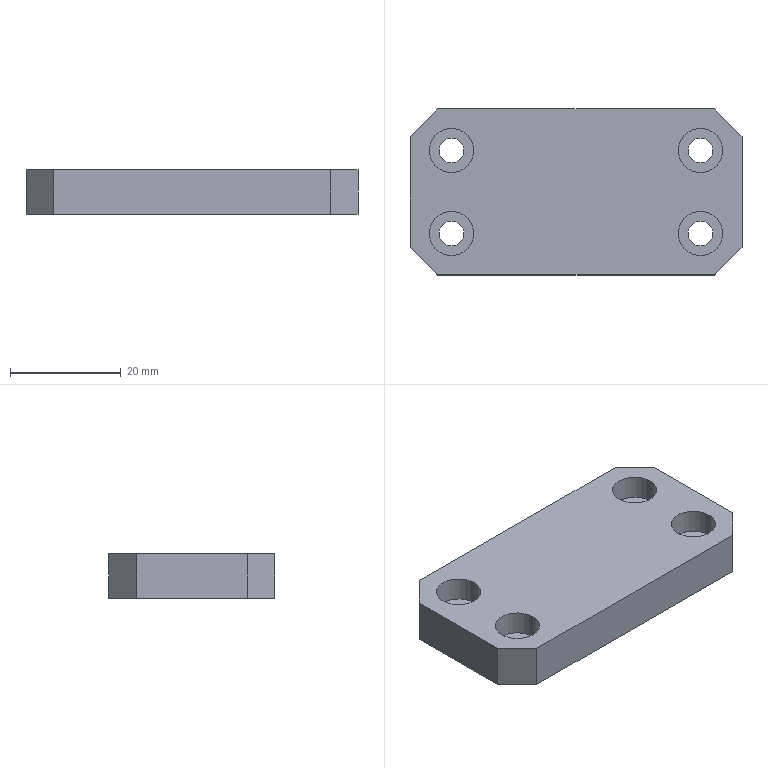Part | SolidWorks | features Chamfer 1, Extrusion 1, HoleWzd 1 | 1 solid | 30 faces | box 60 x 30 x 8 mm | volume 12886 mm3 | cylinder 16 | plane 14 | commonest cylinder face diameters 4.5 x8 8 x8
STEP:
#1=CARTESIAN_POINT('',(-26.5,7.5,3.6));
#2=VERTEX_POINT('',#1);
#3=CARTESIAN_POINT('',(-18.5,7.5,3.6));
#4=VERTEX_POINT('',#3);
#5=CARTESIAN_POINT('',(-22.5,7.5,3.6));
#6=DIRECTION('',(0.,0.,1.));
#7=DIRECTION('',(1.,0.,0.));
#8=AXIS2_PLACEMENT_3D('',#5,#6,#7);
#9=CIRCLE('',#8,4.);
#10=EDGE_CURVE('',#2,#4,#9,.T.);
#11=ORIENTED_EDGE('',*,*,#10,.F.);
#12=CARTESIAN_POINT('',(-26.5,7.5,8.));
#13=VERTEX_POINT('',#12);
#14=CARTESIAN_POINT('',(-26.5,7.5,8.));
#15=DIRECTION('',(0.,0.,1.));
#16=VECTOR('',#15,1000.);
#17=LINE('',#14,#16);
#18=EDGE_CURVE('',#2,#13,#17,.T.);
#19=ORIENTED_EDGE('',*,*,#18,.T.);
#20=CARTESIAN_POINT('',(-18.5,7.5,8.));
#21=VERTEX_POINT('',#20);
#22=CARTESIAN_POINT('',(-22.5,7.5,8.));
#23=DIRECTION('',(0.,0.,1.));
#24=DIRECTION('',(1.,0.,0.));
#25=AXIS2_PLACEMENT_3D('',#22,#23,#24);
#26=CIRCLE('',#25,4.);
#27=EDGE_CURVE('',#13,#21,#26,.T.);
#28=ORIENTED_EDGE('',*,*,#27,.T.);
#29=CARTESIAN_POINT('',(-18.5,7.5,8.));
#30=DIRECTION('',(0.,0.,1.));
#31=VECTOR('',#30,1000.);
#32=LINE('',#29,#31);
#33=EDGE_CURVE('',#4,#21,#32,.T.);
#34=ORIENTED_EDGE('',*,*,#33,.F.);
#35=EDGE_LOOP('',(#11,#19,#28,#34));
#36=FACE_OUTER_BOUND('',#35,.T.);
#37=CARTESIAN_POINT('',(-22.5,7.5,8.));
#38=DIRECTION('',(0.,0.,1.));
#39=DIRECTION('',(1.,0.,0.));
#40=AXIS2_PLACEMENT_3D('',#37,#38,#39);
#41=CYLINDRICAL_SURFACE('',#40,4.);
#42=ADVANCED_FACE('',(#36),#41,.F.);
#43=CARTESIAN_POINT('',(-24.75,7.5,0.));
#44=VERTEX_POINT('',#43);
#45=CARTESIAN_POINT('',(-20.25,7.5,0.));
#46=VERTEX_POINT('',#45);
#47=CARTESIAN_POINT('',(-22.5,7.5,0.));
#48=DIRECTION('',(0.,0.,1.));
#49=DIRECTION('',(1.,0.,0.));
#50=AXIS2_PLACEMENT_3D('',#47,#48,#49);
#51=CIRCLE('',#50,2.25);
#52=EDGE_CURVE('',#44,#46,#51,.T.);
#53=ORIENTED_EDGE('',*,*,#52,.F.);
#54=CARTESIAN_POINT('',(-24.75,7.5,3.6));
#55=VERTEX_POINT('',#54);
#56=CARTESIAN_POINT('',(-24.75,7.5,8.));
#57=DIRECTION('',(0.,0.,1.));
#58=VECTOR('',#57,1000.);
#59=LINE('',#56,#58);
#60=EDGE_CURVE('',#44,#55,#59,.T.);
#61=ORIENTED_EDGE('',*,*,#60,.T.);
#62=CARTESIAN_POINT('',(-20.25,7.5,3.6));
#63=VERTEX_POINT('',#62);
#64=CARTESIAN_POINT('',(-22.5,7.5,3.6));
#65=DIRECTION('',(0.,0.,1.));
#66=DIRECTION('',(1.,0.,0.));
#67=AXIS2_PLACEMENT_3D('',#64,#65,#66);
#68=CIRCLE('',#67,2.25);
#69=EDGE_CURVE('',#55,#63,#68,.T.);
#70=ORIENTED_EDGE('',*,*,#69,.T.);
#71=CARTESIAN_POINT('',(-20.25,7.5,8.));
#72=DIRECTION('',(0.,0.,1.));
#73=VECTOR('',#72,1000.);
#74=LINE('',#71,#73);
#75=EDGE_CURVE('',#46,#63,#74,.T.);
#76=ORIENTED_EDGE('',*,*,#75,.F.);
#77=EDGE_LOOP('',(#53,#61,#70,#76));
#78=FACE_OUTER_BOUND('',#77,.T.);
#79=CARTESIAN_POINT('',(-22.5,7.5,8.));
#80=DIRECTION('',(0.,0.,1.));
#81=DIRECTION('',(1.,0.,0.));
#82=AXIS2_PLACEMENT_3D('',#79,#80,#81);
#83=CYLINDRICAL_SURFACE('',#82,2.25);
#84=ADVANCED_FACE('',(#78),#83,.F.);
#85=CARTESIAN_POINT('',(-26.5,-7.5,3.6));
#86=VERTEX_POINT('',#85);
#87=CARTESIAN_POINT('',(-18.5,-7.5,3.6));
#88=VERTEX_POINT('',#87);
#89=CARTESIAN_POINT('',(-22.5,-7.5,3.6));
#90=DIRECTION('',(0.,0.,1.));
#91=DIRECTION('',(1.,0.,0.));
#92=AXIS2_PLACEMENT_3D('',#89,#90,#91);
#93=CIRCLE('',#92,4.);
#94=EDGE_CURVE('',#86,#88,#93,.T.);
#95=ORIENTED_EDGE('',*,*,#94,.F.);
#96=CARTESIAN_POINT('',(-26.5,-7.5,8.));
#97=VERTEX_POINT('',#96);
#98=CARTESIAN_POINT('',(-26.5,-7.5,8.));
#99=DIRECTION('',(0.,0.,1.));
#100=VECTOR('',#99,1000.);
#101=LINE('',#98,#100);
#102=EDGE_CURVE('',#86,#97,#101,.T.);
#103=ORIENTED_EDGE('',*,*,#102,.T.);
#104=CARTESIAN_POINT('',(-18.5,-7.5,8.));
#105=VERTEX_POINT('',#104);
#106=CARTESIAN_POINT('',(-22.5,-7.5,8.));
#107=DIRECTION('',(0.,0.,1.));
#108=DIRECTION('',(1.,0.,0.));
#109=AXIS2_PLACEMENT_3D('',#106,#107,#108);
#110=CIRCLE('',#109,4.);
#111=EDGE_CURVE('',#97,#105,#110,.T.);
#112=ORIENTED_EDGE('',*,*,#111,.T.);
#113=CARTESIAN_POINT('',(-18.5,-7.5,8.));
#114=DIRECTION('',(0.,0.,1.));
#115=VECTOR('',#114,1000.);
#116=LINE('',#113,#115);
#117=EDGE_CURVE('',#88,#105,#116,.T.);
#118=ORIENTED_EDGE('',*,*,#117,.F.);
#119=EDGE_LOOP('',(#95,#103,#112,#118));
#120=FACE_OUTER_BOUND('',#119,.T.);
#121=CARTESIAN_POINT('',(-22.5,-7.5,8.));
#122=DIRECTION('',(0.,0.,1.));
#123=DIRECTION('',(1.,0.,0.));
#124=AXIS2_PLACEMENT_3D('',#121,#122,#123);
#125=CYLINDRICAL_SURFACE('',#124,4.);
#126=ADVANCED_FACE('',(#120),#125,.F.);
#127=CARTESIAN_POINT('',(-24.75,-7.5,0.));
#128=VERTEX_POINT('',#127);
#129=CARTESIAN_POINT('',(-20.25,-7.5,0.));
#130=VERTEX_POINT('',#129);
#131=CARTESIAN_POINT('',(-22.5,-7.5,0.));
#132=DIRECTION('',(0.,0.,1.));
#133=DIRECTION('',(1.,0.,0.));
#134=AXIS2_PLACEMENT_3D('',#131,#132,#133);
#135=CIRCLE('',#134,2.25);
#136=EDGE_CURVE('',#128,#130,#135,.T.);
#137=ORIENTED_EDGE('',*,*,#136,.F.);
#138=CARTESIAN_POINT('',(-24.75,-7.5,3.6));
#139=VERTEX_POINT('',#138);
#140=CARTESIAN_POINT('',(-24.75,-7.5,8.));
#141=DIRECTION('',(0.,0.,1.));
#142=VECTOR('',#141,1000.);
#143=LINE('',#140,#142);
#144=EDGE_CURVE('',#128,#139,#143,.T.);
#145=ORIENTED_EDGE('',*,*,#144,.T.);
#146=CARTESIAN_POINT('',(-20.25,-7.5,3.6));
#147=VERTEX_POINT('',#146);
#148=CARTESIAN_POINT('',(-22.5,-7.5,3.6));
#149=DIRECTION('',(0.,0.,1.));
#150=DIRECTION('',(1.,0.,0.));
#151=AXIS2_PLACEMENT_3D('',#148,#149,#150);
#152=CIRCLE('',#151,2.25);
#153=EDGE_CURVE('',#139,#147,#152,.T.);
#154=ORIENTED_EDGE('',*,*,#153,.T.);
#155=CARTESIAN_POINT('',(-20.25,-7.5,8.));
#156=DIRECTION('',(0.,0.,1.));
#157=VECTOR('',#156,1000.);
#158=LINE('',#155,#157);
#159=EDGE_CURVE('',#130,#147,#158,.T.);
#160=ORIENTED_EDGE('',*,*,#159,.F.);
#161=EDGE_LOOP('',(#137,#145,#154,#160));
#162=FACE_OUTER_BOUND('',#161,.T.);
#163=CARTESIAN_POINT('',(-22.5,-7.5,8.));
#164=DIRECTION('',(0.,0.,1.));
#165=DIRECTION('',(1.,0.,0.));
#166=AXIS2_PLACEMENT_3D('',#163,#164,#165);
#167=CYLINDRICAL_SURFACE('',#166,2.25);
#168=ADVANCED_FACE('',(#162),#167,.F.);
#169=CARTESIAN_POINT('',(18.5,-7.5,3.6));
#170=VERTEX_POINT('',#169);
#171=CARTESIAN_POINT('',(26.5,-7.5,3.6));
#172=VERTEX_POINT('',#171);
#173=CARTESIAN_POINT('',(22.5,-7.5,3.6));
#174=DIRECTION('',(0.,0.,1.));
#175=DIRECTION('',(1.,0.,0.));
#176=AXIS2_PLACEMENT_3D('',#173,#174,#175);
#177=CIRCLE('',#176,4.);
#178=EDGE_CURVE('',#170,#172,#177,.T.);
#179=ORIENTED_EDGE('',*,*,#178,.F.);
#180=CARTESIAN_POINT('',(18.5,-7.5,8.));
#181=VERTEX_POINT('',#180);
#182=CARTESIAN_POINT('',(18.5,-7.5,8.));
#183=DIRECTION('',(0.,0.,1.));
#184=VECTOR('',#183,1000.);
#185=LINE('',#182,#184);
#186=EDGE_CURVE('',#170,#181,#185,.T.);
#187=ORIENTED_EDGE('',*,*,#186,.T.);
#188=CARTESIAN_POINT('',(26.5,-7.5,8.));
#189=VERTEX_POINT('',#188);
#190=CARTESIAN_POINT('',(22.5,-7.5,8.));
#191=DIRECTION('',(0.,0.,1.));
#192=DIRECTION('',(1.,0.,0.));
#193=AXIS2_PLACEMENT_3D('',#190,#191,#192);
#194=CIRCLE('',#193,4.);
#195=EDGE_CURVE('',#181,#189,#194,.T.);
#196=ORIENTED_EDGE('',*,*,#195,.T.);
#197=CARTESIAN_POINT('',(26.5,-7.5,8.));
#198=DIRECTION('',(0.,0.,1.));
#199=VECTOR('',#198,1000.);
#200=LINE('',#197,#199);
#201=EDGE_CURVE('',#172,#189,#200,.T.);
#202=ORIENTED_EDGE('',*,*,#201,.F.);
#203=EDGE_LOOP('',(#179,#187,#196,#202));
#204=FACE_OUTER_BOUND('',#203,.T.);
#205=CARTESIAN_POINT('',(22.5,-7.5,8.));
#206=DIRECTION('',(0.,0.,1.));
#207=DIRECTION('',(1.,0.,0.));
#208=AXIS2_PLACEMENT_3D('',#205,#206,#207);
#209=CYLINDRICAL_SURFACE('',#208,4.);
#210=ADVANCED_FACE('',(#204),#209,.F.);
#211=CARTESIAN_POINT('',(20.25,-7.5,0.));
#212=VERTEX_POINT('',#211);
#213=CARTESIAN_POINT('',(24.75,-7.5,0.));
#214=VERTEX_POINT('',#213);
#215=CARTESIAN_POINT('',(22.5,-7.5,0.));
#216=DIRECTION('',(0.,0.,1.));
#217=DIRECTION('',(1.,0.,0.));
#218=AXIS2_PLACEMENT_3D('',#215,#216,#217);
#219=CIRCLE('',#218,2.25);
#220=EDGE_CURVE('',#212,#214,#219,.T.);
#221=ORIENTED_EDGE('',*,*,#220,.F.);
#222=CARTESIAN_POINT('',(20.25,-7.5,3.6));
#223=VERTEX_POINT('',#222);
#224=CARTESIAN_POINT('',(20.25,-7.5,8.));
#225=DIRECTION('',(0.,0.,1.));
#226=VECTOR('',#225,1000.);
#227=LINE('',#224,#226);
#228=EDGE_CURVE('',#212,#223,#227,.T.);
#229=ORIENTED_EDGE('',*,*,#228,.T.);
#230=CARTESIAN_POINT('',(24.75,-7.5,3.6));
#231=VERTEX_POINT('',#230);
#232=CARTESIAN_POINT('',(22.5,-7.5,3.6));
#233=DIRECTION('',(0.,0.,1.));
#234=DIRECTION('',(1.,0.,0.));
#235=AXIS2_PLACEMENT_3D('',#232,#233,#234);
#236=CIRCLE('',#235,2.25);
#237=EDGE_CURVE('',#223,#231,#236,.T.);
#238=ORIENTED_EDGE('',*,*,#237,.T.);
#239=CARTESIAN_POINT('',(24.75,-7.5,8.));
#240=DIRECTION('',(0.,0.,1.));
#241=VECTOR('',#240,1000.);
#242=LINE('',#239,#241);
#243=EDGE_CURVE('',#214,#231,#242,.T.);
#244=ORIENTED_EDGE('',*,*,#243,.F.);
#245=EDGE_LOOP('',(#221,#229,#238,#244));
#246=FACE_OUTER_BOUND('',#245,.T.);
#247=CARTESIAN_POINT('',(22.5,-7.5,8.));
#248=DIRECTION('',(0.,0.,1.));
#249=DIRECTION('',(1.,0.,0.));
#250=AXIS2_PLACEMENT_3D('',#247,#248,#249);
#251=CYLINDRICAL_SURFACE('',#250,2.25);
#252=ADVANCED_FACE('',(#246),#251,.F.);
#253=CARTESIAN_POINT('',(18.5,7.5,3.6));
#254=VERTEX_POINT('',#253);
#255=CARTESIAN_POINT('',(26.5,7.5,3.6));
#256=VERTEX_POINT('',#255);
#257=CARTESIAN_POINT('',(22.5,7.5,3.6));
#258=DIRECTION('',(0.,0.,1.));
#259=DIRECTION('',(1.,0.,0.));
#260=AXIS2_PLACEMENT_3D('',#257,#258,#259);
#261=CIRCLE('',#260,4.);
#262=EDGE_CURVE('',#254,#256,#261,.T.);
#263=ORIENTED_EDGE('',*,*,#262,.F.);
#264=CARTESIAN_POINT('',(18.5,7.5,8.));
#265=VERTEX_POINT('',#264);
#266=CARTESIAN_POINT('',(18.5,7.5,8.));
#267=DIRECTION('',(0.,0.,1.));
#268=VECTOR('',#267,1000.);
#269=LINE('',#266,#268);
#270=EDGE_CURVE('',#254,#265,#269,.T.);
#271=ORIENTED_EDGE('',*,*,#270,.T.);
#272=CARTESIAN_POINT('',(26.5,7.5,8.));
#273=VERTEX_POINT('',#272);
#274=CARTESIAN_POINT('',(22.5,7.5,8.));
#275=DIRECTION('',(0.,0.,1.));
#276=DIRECTION('',(1.,0.,0.));
#277=AXIS2_PLACEMENT_3D('',#274,#275,#276);
#278=CIRCLE('',#277,4.);
#279=EDGE_CURVE('',#265,#273,#278,.T.);
#280=ORIENTED_EDGE('',*,*,#279,.T.);
#281=CARTESIAN_POINT('',(26.5,7.5,8.));
#282=DIRECTION('',(0.,0.,1.));
#283=VECTOR('',#282,1000.);
#284=LINE('',#281,#283);
#285=EDGE_CURVE('',#256,#273,#284,.T.);
#286=ORIENTED_EDGE('',*,*,#285,.F.);
#287=EDGE_LOOP('',(#263,#271,#280,#286));
#288=FACE_OUTER_BOUND('',#287,.T.);
#289=CARTESIAN_POINT('',(22.5,7.5,8.));
#290=DIRECTION('',(0.,0.,1.));
#291=DIRECTION('',(1.,0.,0.));
#292=AXIS2_PLACEMENT_3D('',#289,#290,#291);
#293=CYLINDRICAL_SURFACE('',#292,4.);
#294=ADVANCED_FACE('',(#288),#293,.F.);
#295=CARTESIAN_POINT('',(20.25,7.5,0.));
#296=VERTEX_POINT('',#295);
#297=CARTESIAN_POINT('',(24.75,7.5,0.));
#298=VERTEX_POINT('',#297);
#299=CARTESIAN_POINT('',(22.5,7.5,0.));
#300=DIRECTION('',(0.,0.,1.));
#301=DIRECTION('',(1.,0.,0.));
#302=AXIS2_PLACEMENT_3D('',#299,#300,#301);
#303=CIRCLE('',#302,2.25);
#304=EDGE_CURVE('',#296,#298,#303,.T.);
#305=ORIENTED_EDGE('',*,*,#304,.F.);
#306=CARTESIAN_POINT('',(20.25,7.5,3.6));
#307=VERTEX_POINT('',#306);
#308=CARTESIAN_POINT('',(20.25,7.5,8.));
#309=DIRECTION('',(0.,0.,1.));
#310=VECTOR('',#309,1000.);
#311=LINE('',#308,#310);
#312=EDGE_CURVE('',#296,#307,#311,.T.);
#313=ORIENTED_EDGE('',*,*,#312,.T.);
#314=CARTESIAN_POINT('',(24.75,7.5,3.6));
#315=VERTEX_POINT('',#314);
#316=CARTESIAN_POINT('',(22.5,7.5,3.6));
#317=DIRECTION('',(0.,0.,1.));
#318=DIRECTION('',(1.,0.,0.));
#319=AXIS2_PLACEMENT_3D('',#316,#317,#318);
#320=CIRCLE('',#319,2.25);
#321=EDGE_CURVE('',#307,#315,#320,.T.);
#322=ORIENTED_EDGE('',*,*,#321,.T.);
#323=CARTESIAN_POINT('',(24.75,7.5,8.));
#324=DIRECTION('',(0.,0.,1.));
#325=VECTOR('',#324,1000.);
#326=LINE('',#323,#325);
#327=EDGE_CURVE('',#298,#315,#326,.T.);
#328=ORIENTED_EDGE('',*,*,#327,.F.);
#329=EDGE_LOOP('',(#305,#313,#322,#328));
#330=FACE_OUTER_BOUND('',#329,.T.);
#331=CARTESIAN_POINT('',(22.5,7.5,8.));
#332=DIRECTION('',(0.,0.,1.));
#333=DIRECTION('',(1.,0.,0.));
#334=AXIS2_PLACEMENT_3D('',#331,#332,#333);
#335=CYLINDRICAL_SURFACE('',#334,2.25);
#336=ADVANCED_FACE('',(#330),#335,.F.);
#337=CARTESIAN_POINT('',(30.,-10.,0.));
#338=VERTEX_POINT('',#337);
#339=CARTESIAN_POINT('',(30.,10.,0.));
#340=VERTEX_POINT('',#339);
#341=CARTESIAN_POINT('',(30.,15.,0.));
#342=DIRECTION('',(0.,1.,0.));
#343=VECTOR('',#342,1000.);
#344=LINE('',#341,#343);
#345=EDGE_CURVE('',#338,#340,#344,.T.);
#346=ORIENTED_EDGE('',*,*,#345,.T.);
#347=CARTESIAN_POINT('',(30.,10.,8.));
#348=VERTEX_POINT('',#347);
#349=CARTESIAN_POINT('',(30.,10.,8.));
#350=DIRECTION('',(0.,0.,1.));
#351=VECTOR('',#350,1000.);
#352=LINE('',#349,#351);
#353=EDGE_CURVE('',#340,#348,#352,.T.);
#354=ORIENTED_EDGE('',*,*,#353,.T.);
#355=CARTESIAN_POINT('',(30.,-10.,8.));
#356=VERTEX_POINT('',#355);
#357=CARTESIAN_POINT('',(30.,15.,8.));
#358=DIRECTION('',(0.,1.,0.));
#359=VECTOR('',#358,1000.);
#360=LINE('',#357,#359);
#361=EDGE_CURVE('',#356,#348,#360,.T.);
#362=ORIENTED_EDGE('',*,*,#361,.F.);
#363=CARTESIAN_POINT('',(30.,-10.,8.));
#364=DIRECTION('',(0.,0.,-1.));
#365=VECTOR('',#364,1000.);
#366=LINE('',#363,#365);
#367=EDGE_CURVE('',#356,#338,#366,.T.);
#368=ORIENTED_EDGE('',*,*,#367,.T.);
#369=EDGE_LOOP('',(#346,#354,#362,#368));
#370=FACE_OUTER_BOUND('',#369,.T.);
#371=CARTESIAN_POINT('',(30.,15.,8.));
#372=DIRECTION('',(-1.,0.,0.));
#373=DIRECTION('',(0.,0.,1.));
#374=AXIS2_PLACEMENT_3D('',#371,#372,#373);
#375=PLANE('',#374);
#376=ADVANCED_FACE('',(#370),#375,.F.);
#377=CARTESIAN_POINT('',(25.,15.,8.));
#378=VERTEX_POINT('',#377);
#379=CARTESIAN_POINT('',(-25.,15.,8.));
#380=VERTEX_POINT('',#379);
#381=CARTESIAN_POINT('',(-30.,15.,8.));
#382=DIRECTION('',(-1.,0.,0.));
#383=VECTOR('',#382,1000.);
#384=LINE('',#381,#383);
#385=EDGE_CURVE('',#378,#380,#384,.T.);
#386=ORIENTED_EDGE('',*,*,#385,.F.);
#387=CARTESIAN_POINT('',(25.,15.,0.));
#388=VERTEX_POINT('',#387);
#389=CARTESIAN_POINT('',(25.,15.,8.));
#390=DIRECTION('',(0.,0.,-1.));
#391=VECTOR('',#390,1000.);
#392=LINE('',#389,#391);
#393=EDGE_CURVE('',#378,#388,#392,.T.);
#394=ORIENTED_EDGE('',*,*,#393,.T.);
#395=CARTESIAN_POINT('',(-25.,15.,0.));
#396=VERTEX_POINT('',#395);
#397=CARTESIAN_POINT('',(-30.,15.,0.));
#398=DIRECTION('',(-1.,0.,0.));
#399=VECTOR('',#398,1000.);
#400=LINE('',#397,#399);
#401=EDGE_CURVE('',#388,#396,#400,.T.);
#402=ORIENTED_EDGE('',*,*,#401,.T.);
#403=CARTESIAN_POINT('',(-25.,15.,8.));
#404=DIRECTION('',(0.,0.,1.));
#405=VECTOR('',#404,1000.);
#406=LINE('',#403,#405);
#407=EDGE_CURVE('',#396,#380,#406,.T.);
#408=ORIENTED_EDGE('',*,*,#407,.T.);
#409=EDGE_LOOP('',(#386,#394,#402,#408));
#410=FACE_OUTER_BOUND('',#409,.T.);
#411=CARTESIAN_POINT('',(-30.,15.,8.));
#412=DIRECTION('',(0.,-1.,0.));
#413=DIRECTION('',(0.,0.,-1.));
#414=AXIS2_PLACEMENT_3D('',#411,#412,#413);
#415=PLANE('',#414);
#416=ADVANCED_FACE('',(#410),#415,.F.);
#417=CARTESIAN_POINT('',(-30.,10.,0.));
#418=VERTEX_POINT('',#417);
#419=CARTESIAN_POINT('',(-30.,-10.,0.));
#420=VERTEX_POINT('',#419);
#421=CARTESIAN_POINT('',(-30.,15.,0.));
#422=DIRECTION('',(0.,-1.,0.));
#423=VECTOR('',#422,1000.);
#424=LINE('',#421,#423);
#425=EDGE_CURVE('',#418,#420,#424,.T.);
#426=ORIENTED_EDGE('',*,*,#425,.T.);
#427=CARTESIAN_POINT('',(-30.,-10.,8.));
#428=VERTEX_POINT('',#427);
#429=CARTESIAN_POINT('',(-30.,-10.,8.));
#430=DIRECTION('',(0.,0.,1.));
#431=VECTOR('',#430,1000.);
#432=LINE('',#429,#431);
#433=EDGE_CURVE('',#420,#428,#432,.T.);
#434=ORIENTED_EDGE('',*,*,#433,.T.);
#435=CARTESIAN_POINT('',(-30.,10.,8.));
#436=VERTEX_POINT('',#435);
#437=CARTESIAN_POINT('',(-30.,15.,8.));
#438=DIRECTION('',(0.,-1.,0.));
#439=VECTOR('',#438,1000.);
#440=LINE('',#437,#439);
#441=EDGE_CURVE('',#436,#428,#440,.T.);
#442=ORIENTED_EDGE('',*,*,#441,.F.);
#443=CARTESIAN_POINT('',(-30.,10.,8.));
#444=DIRECTION('',(0.,0.,-1.));
#445=VECTOR('',#444,1000.);
#446=LINE('',#443,#445);
#447=EDGE_CURVE('',#436,#418,#446,.T.);
#448=ORIENTED_EDGE('',*,*,#447,.T.);
#449=EDGE_LOOP('',(#426,#434,#442,#448));
#450=FACE_OUTER_BOUND('',#449,.T.);
#451=CARTESIAN_POINT('',(-30.,15.,8.));
#452=DIRECTION('',(1.,0.,0.));
#453=DIRECTION('',(0.,0.,-1.));
#454=AXIS2_PLACEMENT_3D('',#451,#452,#453);
#455=PLANE('',#454);
#456=ADVANCED_FACE('',(#450),#455,.F.);
#457=CARTESIAN_POINT('',(-25.,-15.,0.));
#458=VERTEX_POINT('',#457);
#459=CARTESIAN_POINT('',(25.,-15.,0.));
#460=VERTEX_POINT('',#459);
#461=CARTESIAN_POINT('',(-30.,-15.,0.));
#462=DIRECTION('',(1.,0.,0.));
#463=VECTOR('',#462,1000.);
#464=LINE('',#461,#463);
#465=EDGE_CURVE('',#458,#460,#464,.T.);
#466=ORIENTED_EDGE('',*,*,#465,.T.);
#467=CARTESIAN_POINT('',(25.,-15.,8.));
#468=VERTEX_POINT('',#467);
#469=CARTESIAN_POINT('',(25.,-15.,8.));
#470=DIRECTION('',(0.,0.,1.));
#471=VECTOR('',#470,1000.);
#472=LINE('',#469,#471);
#473=EDGE_CURVE('',#460,#468,#472,.T.);
#474=ORIENTED_EDGE('',*,*,#473,.T.);
#475=CARTESIAN_POINT('',(-25.,-15.,8.));
#476=VERTEX_POINT('',#475);
#477=CARTESIAN_POINT('',(-30.,-15.,8.));
#478=DIRECTION('',(1.,0.,0.));
#479=VECTOR('',#478,1000.);
#480=LINE('',#477,#479);
#481=EDGE_CURVE('',#476,#468,#480,.T.);
#482=ORIENTED_EDGE('',*,*,#481,.F.);
#483=CARTESIAN_POINT('',(-25.,-15.,8.));
#484=DIRECTION('',(0.,0.,-1.));
#485=VECTOR('',#484,1000.);
#486=LINE('',#483,#485);
#487=EDGE_CURVE('',#476,#458,#486,.T.);
#488=ORIENTED_EDGE('',*,*,#487,.T.);
#489=EDGE_LOOP('',(#466,#474,#482,#488));
#490=FACE_OUTER_BOUND('',#489,.T.);
#491=CARTESIAN_POINT('',(-30.,-15.,8.));
#492=DIRECTION('',(0.,1.,0.));
#493=DIRECTION('',(0.,0.,1.));
#494=AXIS2_PLACEMENT_3D('',#491,#492,#493);
#495=PLANE('',#494);
#496=ADVANCED_FACE('',(#490),#495,.F.);
#497=CARTESIAN_POINT('',(-22.5,7.5,8.));
#498=DIRECTION('',(0.,0.,1.));
#499=DIRECTION('',(1.,0.,0.));
#500=AXIS2_PLACEMENT_3D('',#497,#498,#499);
#501=CIRCLE('',#500,4.);
#502=EDGE_CURVE('',#21,#13,#501,.T.);
#503=ORIENTED_EDGE('',*,*,#502,.F.);
#504=ORIENTED_EDGE('',*,*,#27,.F.);
#505=EDGE_LOOP('',(#503,#504));
#506=FACE_BOUND('',#505,.T.);
#507=CARTESIAN_POINT('',(-22.5,-7.5,8.));
#508=DIRECTION('',(0.,0.,1.));
#509=DIRECTION('',(1.,0.,0.));
#510=AXIS2_PLACEMENT_3D('',#507,#508,#509);
#511=CIRCLE('',#510,4.);
#512=EDGE_CURVE('',#105,#97,#511,.T.);
#513=ORIENTED_EDGE('',*,*,#512,.F.);
#514=ORIENTED_EDGE('',*,*,#111,.F.);
#515=EDGE_LOOP('',(#513,#514));
#516=FACE_BOUND('',#515,.T.);
#517=CARTESIAN_POINT('',(22.5,-7.5,8.));
#518=DIRECTION('',(0.,0.,1.));
#519=DIRECTION('',(1.,0.,0.));
#520=AXIS2_PLACEMENT_3D('',#517,#518,#519);
#521=CIRCLE('',#520,4.);
#522=EDGE_CURVE('',#189,#181,#521,.T.);
#523=ORIENTED_EDGE('',*,*,#522,.F.);
#524=ORIENTED_EDGE('',*,*,#195,.F.);
#525=EDGE_LOOP('',(#523,#524));
#526=FACE_BOUND('',#525,.T.);
#527=CARTESIAN_POINT('',(22.5,7.5,8.));
#528=DIRECTION('',(0.,0.,1.));
#529=DIRECTION('',(1.,0.,0.));
#530=AXIS2_PLACEMENT_3D('',#527,#528,#529);
#531=CIRCLE('',#530,4.);
#532=EDGE_CURVE('',#273,#265,#531,.T.);
#533=ORIENTED_EDGE('',*,*,#532,.F.);
#534=ORIENTED_EDGE('',*,*,#279,.F.);
#535=EDGE_LOOP('',(#533,#534));
#536=FACE_BOUND('',#535,.T.);
#537=ORIENTED_EDGE('',*,*,#361,.T.);
#538=CARTESIAN_POINT('',(20.,20.,8.));
#539=DIRECTION('',(-0.7071,0.7071,0.));
#540=VECTOR('',#539,1000.);
#541=LINE('',#538,#540);
#542=EDGE_CURVE('',#348,#378,#541,.T.);
#543=ORIENTED_EDGE('',*,*,#542,.T.);
#544=ORIENTED_EDGE('',*,*,#385,.T.);
#545=CARTESIAN_POINT('',(-20.,20.,8.));
#546=DIRECTION('',(-0.7071,-0.7071,0.));
#547=VECTOR('',#546,1000.);
#548=LINE('',#545,#547);
#549=EDGE_CURVE('',#380,#436,#548,.T.);
#550=ORIENTED_EDGE('',*,*,#549,.T.);
#551=ORIENTED_EDGE('',*,*,#441,.T.);
#552=CARTESIAN_POINT('',(-20.,-20.,8.));
#553=DIRECTION('',(0.7071,-0.7071,0.));
#554=VECTOR('',#553,1000.);
#555=LINE('',#552,#554);
#556=EDGE_CURVE('',#428,#476,#555,.T.);
#557=ORIENTED_EDGE('',*,*,#556,.T.);
#558=ORIENTED_EDGE('',*,*,#481,.T.);
#559=CARTESIAN_POINT('',(20.,-20.,8.));
#560=DIRECTION('',(0.7071,0.7071,0.));
#561=VECTOR('',#560,1000.);
#562=LINE('',#559,#561);
#563=EDGE_CURVE('',#468,#356,#562,.T.);
#564=ORIENTED_EDGE('',*,*,#563,.T.);
#565=EDGE_LOOP('',(#537,#543,#544,#550,#551,#557,#558,#564));
#566=FACE_OUTER_BOUND('',#565,.T.);
#567=CARTESIAN_POINT('',(0.,0.,8.));
#568=DIRECTION('',(0.,0.,1.));
#569=DIRECTION('',(1.,0.,0.));
#570=AXIS2_PLACEMENT_3D('',#567,#568,#569);
#571=PLANE('',#570);
#572=ADVANCED_FACE('',(#506,#516,#526,#536,#566),#571,.T.);
#573=CARTESIAN_POINT('',(-22.5,7.5,0.));
#574=DIRECTION('',(0.,0.,1.));
#575=DIRECTION('',(1.,0.,0.));
#576=AXIS2_PLACEMENT_3D('',#573,#574,#575);
#577=CIRCLE('',#576,2.25);
#578=EDGE_CURVE('',#46,#44,#577,.T.);
#579=ORIENTED_EDGE('',*,*,#578,.T.);
#580=ORIENTED_EDGE('',*,*,#52,.T.);
#581=EDGE_LOOP('',(#579,#580));
#582=FACE_BOUND('',#581,.T.);
#583=CARTESIAN_POINT('',(-22.5,-7.5,0.));
#584=DIRECTION('',(0.,0.,1.));
#585=DIRECTION('',(1.,0.,0.));
#586=AXIS2_PLACEMENT_3D('',#583,#584,#585);
#587=CIRCLE('',#586,2.25);
#588=EDGE_CURVE('',#130,#128,#587,.T.);
#589=ORIENTED_EDGE('',*,*,#588,.T.);
#590=ORIENTED_EDGE('',*,*,#136,.T.);
#591=EDGE_LOOP('',(#589,#590));
#592=FACE_BOUND('',#591,.T.);
#593=CARTESIAN_POINT('',(22.5,-7.5,0.));
#594=DIRECTION('',(0.,0.,1.));
#595=DIRECTION('',(1.,0.,0.));
#596=AXIS2_PLACEMENT_3D('',#593,#594,#595);
#597=CIRCLE('',#596,2.25);
#598=EDGE_CURVE('',#214,#212,#597,.T.);
#599=ORIENTED_EDGE('',*,*,#598,.T.);
#600=ORIENTED_EDGE('',*,*,#220,.T.);
#601=EDGE_LOOP('',(#599,#600));
#602=FACE_BOUND('',#601,.T.);
#603=CARTESIAN_POINT('',(22.5,7.5,0.));
#604=DIRECTION('',(0.,0.,1.));
#605=DIRECTION('',(1.,0.,0.));
#606=AXIS2_PLACEMENT_3D('',#603,#604,#605);
#607=CIRCLE('',#606,2.25);
#608=EDGE_CURVE('',#298,#296,#607,.T.);
#609=ORIENTED_EDGE('',*,*,#608,.T.);
#610=ORIENTED_EDGE('',*,*,#304,.T.);
#611=EDGE_LOOP('',(#609,#610));
#612=FACE_BOUND('',#611,.T.);
#613=ORIENTED_EDGE('',*,*,#401,.F.);
#614=CARTESIAN_POINT('',(25.,15.,0.));
#615=DIRECTION('',(0.7071,-0.7071,0.));
#616=VECTOR('',#615,1000.);
#617=LINE('',#614,#616);
#618=EDGE_CURVE('',#388,#340,#617,.T.);
#619=ORIENTED_EDGE('',*,*,#618,.T.);
#620=ORIENTED_EDGE('',*,*,#345,.F.);
#621=CARTESIAN_POINT('',(30.,-10.,0.));
#622=DIRECTION('',(-0.7071,-0.7071,0.));
#623=VECTOR('',#622,1000.);
#624=LINE('',#621,#623);
#625=EDGE_CURVE('',#338,#460,#624,.T.);
#626=ORIENTED_EDGE('',*,*,#625,.T.);
#627=ORIENTED_EDGE('',*,*,#465,.F.);
#628=CARTESIAN_POINT('',(-25.,-15.,0.));
#629=DIRECTION('',(-0.7071,0.7071,0.));
#630=VECTOR('',#629,1000.);
#631=LINE('',#628,#630);
#632=EDGE_CURVE('',#458,#420,#631,.T.);
#633=ORIENTED_EDGE('',*,*,#632,.T.);
#634=ORIENTED_EDGE('',*,*,#425,.F.);
#635=CARTESIAN_POINT('',(-30.,10.,0.));
#636=DIRECTION('',(0.7071,0.7071,0.));
#637=VECTOR('',#636,1000.);
#638=LINE('',#635,#637);
#639=EDGE_CURVE('',#418,#396,#638,.T.);
#640=ORIENTED_EDGE('',*,*,#639,.T.);
#641=EDGE_LOOP('',(#613,#619,#620,#626,#627,#633,#634,#640));
#642=FACE_OUTER_BOUND('',#641,.T.);
#643=CARTESIAN_POINT('',(0.,0.,0.));
#644=DIRECTION('',(0.,0.,1.));
#645=DIRECTION('',(1.,0.,0.));
#646=AXIS2_PLACEMENT_3D('',#643,#644,#645);
#647=PLANE('',#646);
#648=ADVANCED_FACE('',(#582,#592,#602,#612,#642),#647,.F.);
#649=ORIENTED_EDGE('',*,*,#312,.F.);
#650=ORIENTED_EDGE('',*,*,#608,.F.);
#651=ORIENTED_EDGE('',*,*,#327,.T.);
#652=CARTESIAN_POINT('',(22.5,7.5,3.6));
#653=DIRECTION('',(0.,0.,1.));
#654=DIRECTION('',(1.,0.,0.));
#655=AXIS2_PLACEMENT_3D('',#652,#653,#654);
#656=CIRCLE('',#655,2.25);
#657=EDGE_CURVE('',#315,#307,#656,.T.);
#658=ORIENTED_EDGE('',*,*,#657,.T.);
#659=EDGE_LOOP('',(#649,#650,#651,#658));
#660=FACE_OUTER_BOUND('',#659,.T.);
#661=CARTESIAN_POINT('',(22.5,7.5,8.));
#662=DIRECTION('',(0.,0.,1.));
#663=DIRECTION('',(1.,0.,0.));
#664=AXIS2_PLACEMENT_3D('',#661,#662,#663);
#665=CYLINDRICAL_SURFACE('',#664,2.25);
#666=ADVANCED_FACE('',(#660),#665,.F.);
#667=ORIENTED_EDGE('',*,*,#657,.F.);
#668=ORIENTED_EDGE('',*,*,#321,.F.);
#669=EDGE_LOOP('',(#667,#668));
#670=FACE_BOUND('',#669,.T.);
#671=CARTESIAN_POINT('',(22.5,7.5,3.6));
#672=DIRECTION('',(0.,0.,1.));
#673=DIRECTION('',(1.,0.,0.));
#674=AXIS2_PLACEMENT_3D('',#671,#672,#673);
#675=CIRCLE('',#674,4.);
#676=EDGE_CURVE('',#256,#254,#675,.T.);
#677=ORIENTED_EDGE('',*,*,#676,.T.);
#678=ORIENTED_EDGE('',*,*,#262,.T.);
#679=EDGE_LOOP('',(#677,#678));
#680=FACE_OUTER_BOUND('',#679,.T.);
#681=CARTESIAN_POINT('',(24.75,7.5,3.6));
#682=DIRECTION('',(0.,0.,-1.));
#683=DIRECTION('',(-1.,0.,0.));
#684=AXIS2_PLACEMENT_3D('',#681,#682,#683);
#685=PLANE('',#684);
#686=ADVANCED_FACE('',(#670,#680),#685,.F.);
#687=ORIENTED_EDGE('',*,*,#270,.F.);
#688=ORIENTED_EDGE('',*,*,#676,.F.);
#689=ORIENTED_EDGE('',*,*,#285,.T.);
#690=ORIENTED_EDGE('',*,*,#532,.T.);
#691=EDGE_LOOP('',(#687,#688,#689,#690));
#692=FACE_OUTER_BOUND('',#691,.T.);
#693=CARTESIAN_POINT('',(22.5,7.5,8.));
#694=DIRECTION('',(0.,0.,1.));
#695=DIRECTION('',(1.,0.,0.));
#696=AXIS2_PLACEMENT_3D('',#693,#694,#695);
#697=CYLINDRICAL_SURFACE('',#696,4.);
#698=ADVANCED_FACE('',(#692),#697,.F.);
#699=ORIENTED_EDGE('',*,*,#228,.F.);
#700=ORIENTED_EDGE('',*,*,#598,.F.);
#701=ORIENTED_EDGE('',*,*,#243,.T.);
#702=CARTESIAN_POINT('',(22.5,-7.5,3.6));
#703=DIRECTION('',(0.,0.,1.));
#704=DIRECTION('',(1.,0.,0.));
#705=AXIS2_PLACEMENT_3D('',#702,#703,#704);
#706=CIRCLE('',#705,2.25);
#707=EDGE_CURVE('',#231,#223,#706,.T.);
#708=ORIENTED_EDGE('',*,*,#707,.T.);
#709=EDGE_LOOP('',(#699,#700,#701,#708));
#710=FACE_OUTER_BOUND('',#709,.T.);
#711=CARTESIAN_POINT('',(22.5,-7.5,8.));
#712=DIRECTION('',(0.,0.,1.));
#713=DIRECTION('',(1.,0.,0.));
#714=AXIS2_PLACEMENT_3D('',#711,#712,#713);
#715=CYLINDRICAL_SURFACE('',#714,2.25);
#716=ADVANCED_FACE('',(#710),#715,.F.);
#717=ORIENTED_EDGE('',*,*,#707,.F.);
#718=ORIENTED_EDGE('',*,*,#237,.F.);
#719=EDGE_LOOP('',(#717,#718));
#720=FACE_BOUND('',#719,.T.);
#721=CARTESIAN_POINT('',(22.5,-7.5,3.6));
#722=DIRECTION('',(0.,0.,1.));
#723=DIRECTION('',(1.,0.,0.));
#724=AXIS2_PLACEMENT_3D('',#721,#722,#723);
#725=CIRCLE('',#724,4.);
#726=EDGE_CURVE('',#172,#170,#725,.T.);
#727=ORIENTED_EDGE('',*,*,#726,.T.);
#728=ORIENTED_EDGE('',*,*,#178,.T.);
#729=EDGE_LOOP('',(#727,#728));
#730=FACE_OUTER_BOUND('',#729,.T.);
#731=CARTESIAN_POINT('',(24.75,-7.5,3.6));
#732=DIRECTION('',(0.,0.,-1.));
#733=DIRECTION('',(-1.,0.,0.));
#734=AXIS2_PLACEMENT_3D('',#731,#732,#733);
#735=PLANE('',#734);
#736=ADVANCED_FACE('',(#720,#730),#735,.F.);
#737=ORIENTED_EDGE('',*,*,#186,.F.);
#738=ORIENTED_EDGE('',*,*,#726,.F.);
#739=ORIENTED_EDGE('',*,*,#201,.T.);
#740=ORIENTED_EDGE('',*,*,#522,.T.);
#741=EDGE_LOOP('',(#737,#738,#739,#740));
#742=FACE_OUTER_BOUND('',#741,.T.);
#743=CARTESIAN_POINT('',(22.5,-7.5,8.));
#744=DIRECTION('',(0.,0.,1.));
#745=DIRECTION('',(1.,0.,0.));
#746=AXIS2_PLACEMENT_3D('',#743,#744,#745);
#747=CYLINDRICAL_SURFACE('',#746,4.);
#748=ADVANCED_FACE('',(#742),#747,.F.);
#749=ORIENTED_EDGE('',*,*,#144,.F.);
#750=ORIENTED_EDGE('',*,*,#588,.F.);
#751=ORIENTED_EDGE('',*,*,#159,.T.);
#752=CARTESIAN_POINT('',(-22.5,-7.5,3.6));
#753=DIRECTION('',(0.,0.,1.));
#754=DIRECTION('',(1.,0.,0.));
#755=AXIS2_PLACEMENT_3D('',#752,#753,#754);
#756=CIRCLE('',#755,2.25);
#757=EDGE_CURVE('',#147,#139,#756,.T.);
#758=ORIENTED_EDGE('',*,*,#757,.T.);
#759=EDGE_LOOP('',(#749,#750,#751,#758));
#760=FACE_OUTER_BOUND('',#759,.T.);
#761=CARTESIAN_POINT('',(-22.5,-7.5,8.));
#762=DIRECTION('',(0.,0.,1.));
#763=DIRECTION('',(1.,0.,0.));
#764=AXIS2_PLACEMENT_3D('',#761,#762,#763);
#765=CYLINDRICAL_SURFACE('',#764,2.25);
#766=ADVANCED_FACE('',(#760),#765,.F.);
#767=ORIENTED_EDGE('',*,*,#757,.F.);
#768=ORIENTED_EDGE('',*,*,#153,.F.);
#769=EDGE_LOOP('',(#767,#768));
#770=FACE_BOUND('',#769,.T.);
#771=CARTESIAN_POINT('',(-22.5,-7.5,3.6));
#772=DIRECTION('',(0.,0.,1.));
#773=DIRECTION('',(1.,0.,0.));
#774=AXIS2_PLACEMENT_3D('',#771,#772,#773);
#775=CIRCLE('',#774,4.);
#776=EDGE_CURVE('',#88,#86,#775,.T.);
#777=ORIENTED_EDGE('',*,*,#776,.T.);
#778=ORIENTED_EDGE('',*,*,#94,.T.);
#779=EDGE_LOOP('',(#777,#778));
#780=FACE_OUTER_BOUND('',#779,.T.);
#781=CARTESIAN_POINT('',(-20.25,-7.5,3.6));
#782=DIRECTION('',(0.,0.,-1.));
#783=DIRECTION('',(-1.,0.,0.));
#784=AXIS2_PLACEMENT_3D('',#781,#782,#783);
#785=PLANE('',#784);
#786=ADVANCED_FACE('',(#770,#780),#785,.F.);
#787=ORIENTED_EDGE('',*,*,#102,.F.);
#788=ORIENTED_EDGE('',*,*,#776,.F.);
#789=ORIENTED_EDGE('',*,*,#117,.T.);
#790=ORIENTED_EDGE('',*,*,#512,.T.);
#791=EDGE_LOOP('',(#787,#788,#789,#790));
#792=FACE_OUTER_BOUND('',#791,.T.);
#793=CARTESIAN_POINT('',(-22.5,-7.5,8.));
#794=DIRECTION('',(0.,0.,1.));
#795=DIRECTION('',(1.,0.,0.));
#796=AXIS2_PLACEMENT_3D('',#793,#794,#795);
#797=CYLINDRICAL_SURFACE('',#796,4.);
#798=ADVANCED_FACE('',(#792),#797,.F.);
#799=ORIENTED_EDGE('',*,*,#60,.F.);
#800=ORIENTED_EDGE('',*,*,#578,.F.);
#801=ORIENTED_EDGE('',*,*,#75,.T.);
#802=CARTESIAN_POINT('',(-22.5,7.5,3.6));
#803=DIRECTION('',(0.,0.,1.));
#804=DIRECTION('',(1.,0.,0.));
#805=AXIS2_PLACEMENT_3D('',#802,#803,#804);
#806=CIRCLE('',#805,2.25);
#807=EDGE_CURVE('',#63,#55,#806,.T.);
#808=ORIENTED_EDGE('',*,*,#807,.T.);
#809=EDGE_LOOP('',(#799,#800,#801,#808));
#810=FACE_OUTER_BOUND('',#809,.T.);
#811=CARTESIAN_POINT('',(-22.5,7.5,8.));
#812=DIRECTION('',(0.,0.,1.));
#813=DIRECTION('',(1.,0.,0.));
#814=AXIS2_PLACEMENT_3D('',#811,#812,#813);
#815=CYLINDRICAL_SURFACE('',#814,2.25);
#816=ADVANCED_FACE('',(#810),#815,.F.);
#817=ORIENTED_EDGE('',*,*,#807,.F.);
#818=ORIENTED_EDGE('',*,*,#69,.F.);
#819=EDGE_LOOP('',(#817,#818));
#820=FACE_BOUND('',#819,.T.);
#821=CARTESIAN_POINT('',(-22.5,7.5,3.6));
#822=DIRECTION('',(0.,0.,1.));
#823=DIRECTION('',(1.,0.,0.));
#824=AXIS2_PLACEMENT_3D('',#821,#822,#823);
#825=CIRCLE('',#824,4.);
#826=EDGE_CURVE('',#4,#2,#825,.T.);
#827=ORIENTED_EDGE('',*,*,#826,.T.);
#828=ORIENTED_EDGE('',*,*,#10,.T.);
#829=EDGE_LOOP('',(#827,#828));
#830=FACE_OUTER_BOUND('',#829,.T.);
#831=CARTESIAN_POINT('',(-20.25,7.5,3.6));
#832=DIRECTION('',(0.,0.,-1.));
#833=DIRECTION('',(-1.,0.,0.));
#834=AXIS2_PLACEMENT_3D('',#831,#832,#833);
#835=PLANE('',#834);
#836=ADVANCED_FACE('',(#820,#830),#835,.F.);
#837=ORIENTED_EDGE('',*,*,#18,.F.);
#838=ORIENTED_EDGE('',*,*,#826,.F.);
#839=ORIENTED_EDGE('',*,*,#33,.T.);
#840=ORIENTED_EDGE('',*,*,#502,.T.);
#841=EDGE_LOOP('',(#837,#838,#839,#840));
#842=FACE_OUTER_BOUND('',#841,.T.);
#843=CARTESIAN_POINT('',(-22.5,7.5,8.));
#844=DIRECTION('',(0.,0.,1.));
#845=DIRECTION('',(1.,0.,0.));
#846=AXIS2_PLACEMENT_3D('',#843,#844,#845);
#847=CYLINDRICAL_SURFACE('',#846,4.);
#848=ADVANCED_FACE('',(#842),#847,.F.);
#849=ORIENTED_EDGE('',*,*,#542,.F.);
#850=ORIENTED_EDGE('',*,*,#353,.F.);
#851=ORIENTED_EDGE('',*,*,#618,.F.);
#852=ORIENTED_EDGE('',*,*,#393,.F.);
#853=EDGE_LOOP('',(#849,#850,#851,#852));
#854=FACE_OUTER_BOUND('',#853,.T.);
#855=CARTESIAN_POINT('',(25.,15.,8.));
#856=DIRECTION('',(-0.7071,-0.7071,0.));
#857=DIRECTION('',(0.,0.,-1.));
#858=AXIS2_PLACEMENT_3D('',#855,#856,#857);
#859=PLANE('',#858);
#860=ADVANCED_FACE('',(#854),#859,.F.);
#861=ORIENTED_EDGE('',*,*,#563,.F.);
#862=ORIENTED_EDGE('',*,*,#473,.F.);
#863=ORIENTED_EDGE('',*,*,#625,.F.);
#864=ORIENTED_EDGE('',*,*,#367,.F.);
#865=EDGE_LOOP('',(#861,#862,#863,#864));
#866=FACE_OUTER_BOUND('',#865,.T.);
#867=CARTESIAN_POINT('',(30.,-10.,8.));
#868=DIRECTION('',(-0.7071,0.7071,0.));
#869=DIRECTION('',(0.,0.,-1.));
#870=AXIS2_PLACEMENT_3D('',#867,#868,#869);
#871=PLANE('',#870);
#872=ADVANCED_FACE('',(#866),#871,.F.);
#873=ORIENTED_EDGE('',*,*,#556,.F.);
#874=ORIENTED_EDGE('',*,*,#433,.F.);
#875=ORIENTED_EDGE('',*,*,#632,.F.);
#876=ORIENTED_EDGE('',*,*,#487,.F.);
#877=EDGE_LOOP('',(#873,#874,#875,#876));
#878=FACE_OUTER_BOUND('',#877,.T.);
#879=CARTESIAN_POINT('',(-25.,-15.,8.));
#880=DIRECTION('',(0.7071,0.7071,0.));
#881=DIRECTION('',(0.,0.,-1.));
#882=AXIS2_PLACEMENT_3D('',#879,#880,#881);
#883=PLANE('',#882);
#884=ADVANCED_FACE('',(#878),#883,.F.);
#885=ORIENTED_EDGE('',*,*,#549,.F.);
#886=ORIENTED_EDGE('',*,*,#407,.F.);
#887=ORIENTED_EDGE('',*,*,#639,.F.);
#888=ORIENTED_EDGE('',*,*,#447,.F.);
#889=EDGE_LOOP('',(#885,#886,#887,#888));
#890=FACE_OUTER_BOUND('',#889,.T.);
#891=CARTESIAN_POINT('',(-30.,10.,8.));
#892=DIRECTION('',(0.7071,-0.7071,0.));
#893=DIRECTION('',(0.,0.,-1.));
#894=AXIS2_PLACEMENT_3D('',#891,#892,#893);
#895=PLANE('',#894);
#896=ADVANCED_FACE('',(#890),#895,.F.);
#897=CLOSED_SHELL('',(#42,#84,#126,#168,#210,#252,#294,#336,#376,#416,#456,#496,#572,#648,#666,#686,#698,#716,#736,#748,#766,#786,#798,#816,#836,#848,#860,#872,#884,#896));
#898=MANIFOLD_SOLID_BREP('',#897);
#899=CARTESIAN_POINT('',(0.,0.,0.));
#900=DIRECTION('',(0.,0.,1.));
#901=DIRECTION('',(1.,0.,0.));
#902=AXIS2_PLACEMENT_3D('',#899,#900,#901);
#903=(LENGTH_UNIT()NAMED_UNIT(*)SI_UNIT(.MILLI.,.METRE.));
#904=UNCERTAINTY_MEASURE_WITH_UNIT(LENGTH_MEASURE(0.00001),#903,'','');
#905=(NAMED_UNIT(*)PLANE_ANGLE_UNIT()SI_UNIT($,.RADIAN.));
#906=(NAMED_UNIT(*)SI_UNIT($,.STERADIAN.)SOLID_ANGLE_UNIT());
#907=(GEOMETRIC_REPRESENTATION_CONTEXT(3)GLOBAL_UNCERTAINTY_ASSIGNED_CONTEXT((#904))GLOBAL_UNIT_ASSIGNED_CONTEXT((#903,#905,#906))REPRESENTATION_CONTEXT('',''));
#908=ADVANCED_BREP_SHAPE_REPRESENTATION('',(#898,#902),#907);